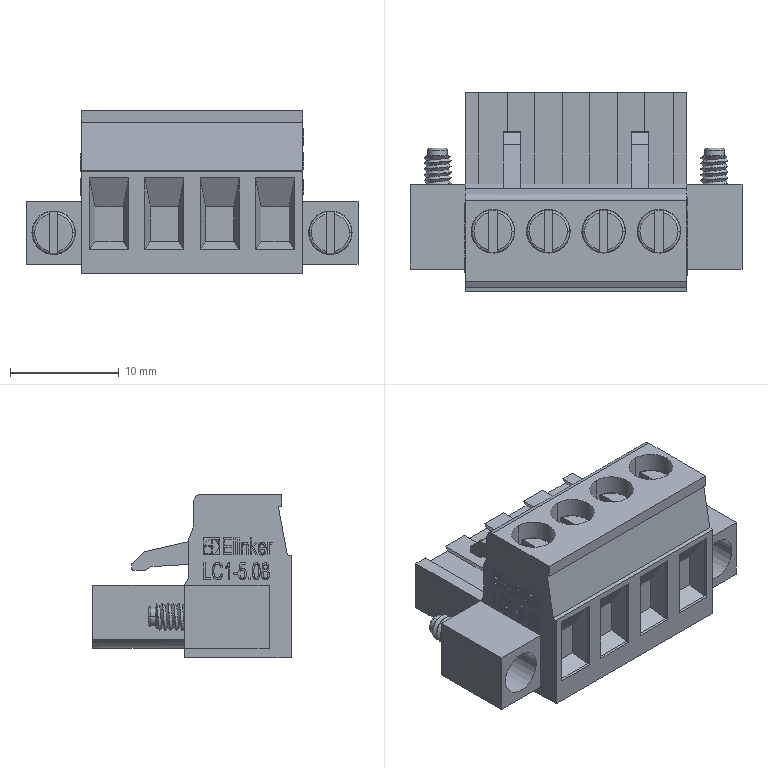Part | NX | features BREP 9 | 9 solids | 2748 faces | box 30.48 x 18.2 x 15 mm | volume 3734 mm3 | plane 2429 | spline 134 | cylinder 117 | torus 56 | cone 12 | commonest cylinder face diameters 2.5 x22 3.9 x12 4 x12 3 x8 0.443 x6 0.093 x4